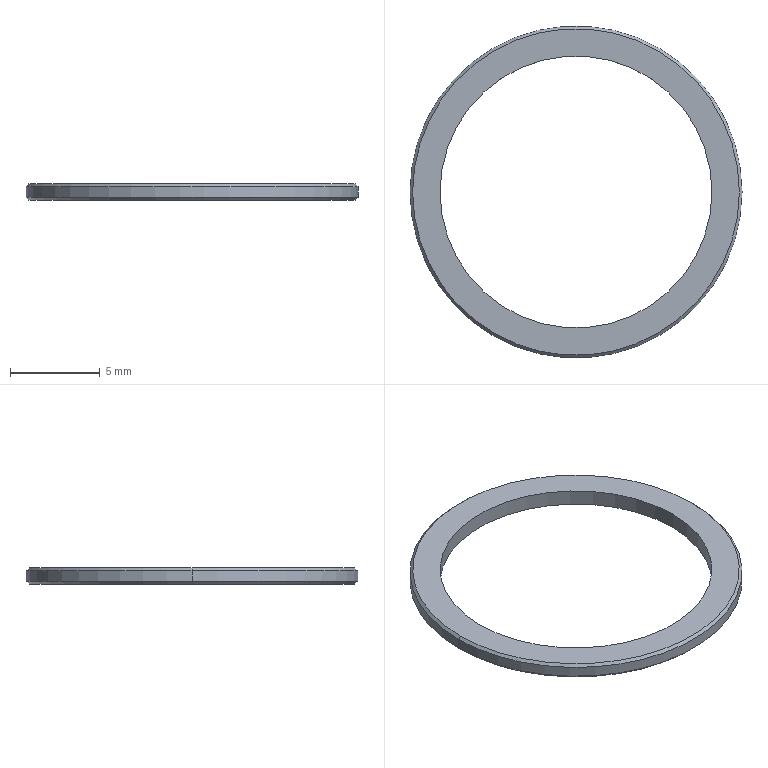Part | STEP file | ARANDELA INT. RODAJA | 1 solid | 10 faces | box 18.5 x 18.5 x 0.9 mm | volume 78.382 mm3 | cone 4 | cylinder 4 | plane 2 | commonest cylinder face diameters 15.15 x2 18.5 x2
STEP:
#1=CARTESIAN_POINT('',(9.1,0.,0.9));
#2=VERTEX_POINT('',#1);
#3=CARTESIAN_POINT('',(-9.1,0.,0.9));
#4=VERTEX_POINT('',#3);
#5=CARTESIAN_POINT('',(0.,0.,0.9));
#6=DIRECTION('',(0.,0.,1.));
#7=DIRECTION('',(1.,0.,0.));
#8=AXIS2_PLACEMENT_3D('',#5,#6,#7);
#9=CIRCLE('',#8,9.1);
#10=EDGE_CURVE('',#2,#4,#9,.T.);
#11=ORIENTED_EDGE('',*,*,#10,.F.);
#12=CARTESIAN_POINT('',(9.25,0.,0.75));
#13=VERTEX_POINT('',#12);
#14=CARTESIAN_POINT('',(9.1,0.,0.9));
#15=DIRECTION('',(0.7071,0.,-0.7071));
#16=VECTOR('',#15,1000.);
#17=LINE('',#14,#16);
#18=EDGE_CURVE('',#2,#13,#17,.T.);
#19=ORIENTED_EDGE('',*,*,#18,.T.);
#20=CARTESIAN_POINT('',(-9.25,0.,0.75));
#21=VERTEX_POINT('',#20);
#22=CARTESIAN_POINT('',(0.,0.,0.75));
#23=DIRECTION('',(0.,0.,-1.));
#24=DIRECTION('',(1.,0.,0.));
#25=AXIS2_PLACEMENT_3D('',#22,#23,#24);
#26=CIRCLE('',#25,9.25);
#27=EDGE_CURVE('',#21,#13,#26,.T.);
#28=ORIENTED_EDGE('',*,*,#27,.F.);
#29=CARTESIAN_POINT('',(-9.1,0.,0.9));
#30=DIRECTION('',(-0.7071,0.,-0.7071));
#31=VECTOR('',#30,1000.);
#32=LINE('',#29,#31);
#33=EDGE_CURVE('',#4,#21,#32,.T.);
#34=ORIENTED_EDGE('',*,*,#33,.F.);
#35=EDGE_LOOP('',(#11,#19,#28,#34));
#36=FACE_OUTER_BOUND('',#35,.T.);
#37=CARTESIAN_POINT('',(0.,0.,0.9));
#38=DIRECTION('',(0.,0.,-1.));
#39=DIRECTION('',(-1.,0.,0.));
#40=AXIS2_PLACEMENT_3D('',#37,#38,#39);
#41=CONICAL_SURFACE('',#40,9.1,0.7854);
#42=ADVANCED_FACE('',(#36),#41,.T.);
#43=CARTESIAN_POINT('',(-9.1,0.,0.));
#44=VERTEX_POINT('',#43);
#45=CARTESIAN_POINT('',(9.1,0.,0.));
#46=VERTEX_POINT('',#45);
#47=CARTESIAN_POINT('',(0.,0.,0.));
#48=DIRECTION('',(0.,0.,-1.));
#49=DIRECTION('',(1.,0.,0.));
#50=AXIS2_PLACEMENT_3D('',#47,#48,#49);
#51=CIRCLE('',#50,9.1);
#52=EDGE_CURVE('',#44,#46,#51,.T.);
#53=ORIENTED_EDGE('',*,*,#52,.F.);
#54=CARTESIAN_POINT('',(-9.25,0.,0.15));
#55=VERTEX_POINT('',#54);
#56=CARTESIAN_POINT('',(-9.25,0.,0.15));
#57=DIRECTION('',(-0.7071,0.,0.7071));
#58=VECTOR('',#57,1000.);
#59=LINE('',#56,#58);
#60=EDGE_CURVE('',#44,#55,#59,.T.);
#61=ORIENTED_EDGE('',*,*,#60,.T.);
#62=CARTESIAN_POINT('',(9.25,0.,0.15));
#63=VERTEX_POINT('',#62);
#64=CARTESIAN_POINT('',(0.,0.,0.15));
#65=DIRECTION('',(0.,0.,1.));
#66=DIRECTION('',(1.,0.,0.));
#67=AXIS2_PLACEMENT_3D('',#64,#65,#66);
#68=CIRCLE('',#67,9.25);
#69=EDGE_CURVE('',#63,#55,#68,.T.);
#70=ORIENTED_EDGE('',*,*,#69,.F.);
#71=CARTESIAN_POINT('',(9.25,0.,0.15));
#72=DIRECTION('',(0.7071,0.,0.7071));
#73=VECTOR('',#72,1000.);
#74=LINE('',#71,#73);
#75=EDGE_CURVE('',#46,#63,#74,.T.);
#76=ORIENTED_EDGE('',*,*,#75,.F.);
#77=EDGE_LOOP('',(#53,#61,#70,#76));
#78=FACE_OUTER_BOUND('',#77,.T.);
#79=CARTESIAN_POINT('',(0.,0.,0.15));
#80=DIRECTION('',(0.,0.,1.));
#81=DIRECTION('',(1.,0.,0.));
#82=AXIS2_PLACEMENT_3D('',#79,#80,#81);
#83=CONICAL_SURFACE('',#82,9.25,0.7854);
#84=ADVANCED_FACE('',(#78),#83,.T.);
#85=CARTESIAN_POINT('',(-7.575,0.,0.9));
#86=VERTEX_POINT('',#85);
#87=CARTESIAN_POINT('',(7.575,0.,0.9));
#88=VERTEX_POINT('',#87);
#89=CARTESIAN_POINT('',(0.,0.,0.9));
#90=DIRECTION('',(0.,0.,1.));
#91=DIRECTION('',(1.,0.,0.));
#92=AXIS2_PLACEMENT_3D('',#89,#90,#91);
#93=CIRCLE('',#92,7.575);
#94=EDGE_CURVE('',#86,#88,#93,.T.);
#95=ORIENTED_EDGE('',*,*,#94,.T.);
#96=CARTESIAN_POINT('',(7.575,0.,0.));
#97=VERTEX_POINT('',#96);
#98=CARTESIAN_POINT('',(7.575,0.,0.9));
#99=DIRECTION('',(0.,0.,-1.));
#100=VECTOR('',#99,1000.);
#101=LINE('',#98,#100);
#102=EDGE_CURVE('',#88,#97,#101,.T.);
#103=ORIENTED_EDGE('',*,*,#102,.T.);
#104=CARTESIAN_POINT('',(-7.575,0.,0.));
#105=VERTEX_POINT('',#104);
#106=CARTESIAN_POINT('',(0.,0.,0.));
#107=DIRECTION('',(0.,0.,1.));
#108=DIRECTION('',(1.,0.,0.));
#109=AXIS2_PLACEMENT_3D('',#106,#107,#108);
#110=CIRCLE('',#109,7.575);
#111=EDGE_CURVE('',#105,#97,#110,.T.);
#112=ORIENTED_EDGE('',*,*,#111,.F.);
#113=CARTESIAN_POINT('',(-7.575,0.,0.9));
#114=DIRECTION('',(0.,0.,-1.));
#115=VECTOR('',#114,1000.);
#116=LINE('',#113,#115);
#117=EDGE_CURVE('',#86,#105,#116,.T.);
#118=ORIENTED_EDGE('',*,*,#117,.F.);
#119=EDGE_LOOP('',(#95,#103,#112,#118));
#120=FACE_OUTER_BOUND('',#119,.T.);
#121=CARTESIAN_POINT('',(0.,0.,0.9));
#122=DIRECTION('',(0.,0.,-1.));
#123=DIRECTION('',(-1.,0.,0.));
#124=AXIS2_PLACEMENT_3D('',#121,#122,#123);
#125=CYLINDRICAL_SURFACE('',#124,7.575);
#126=ADVANCED_FACE('',(#120),#125,.F.);
#127=ORIENTED_EDGE('',*,*,#27,.T.);
#128=CARTESIAN_POINT('',(9.25,0.,0.9));
#129=DIRECTION('',(0.,0.,-1.));
#130=VECTOR('',#129,1000.);
#131=LINE('',#128,#130);
#132=EDGE_CURVE('',#13,#63,#131,.T.);
#133=ORIENTED_EDGE('',*,*,#132,.T.);
#134=ORIENTED_EDGE('',*,*,#69,.T.);
#135=CARTESIAN_POINT('',(-9.25,0.,0.9));
#136=DIRECTION('',(0.,0.,-1.));
#137=VECTOR('',#136,1000.);
#138=LINE('',#135,#137);
#139=EDGE_CURVE('',#21,#55,#138,.T.);
#140=ORIENTED_EDGE('',*,*,#139,.F.);
#141=EDGE_LOOP('',(#127,#133,#134,#140));
#142=FACE_OUTER_BOUND('',#141,.T.);
#143=CARTESIAN_POINT('',(0.,0.,0.9));
#144=DIRECTION('',(0.,0.,-1.));
#145=DIRECTION('',(-1.,0.,0.));
#146=AXIS2_PLACEMENT_3D('',#143,#144,#145);
#147=CYLINDRICAL_SURFACE('',#146,9.25);
#148=ADVANCED_FACE('',(#142),#147,.T.);
#149=CARTESIAN_POINT('',(0.,0.,0.9));
#150=DIRECTION('',(0.,0.,1.));
#151=DIRECTION('',(1.,0.,0.));
#152=AXIS2_PLACEMENT_3D('',#149,#150,#151);
#153=CIRCLE('',#152,9.1);
#154=EDGE_CURVE('',#4,#2,#153,.T.);
#155=ORIENTED_EDGE('',*,*,#154,.T.);
#156=ORIENTED_EDGE('',*,*,#10,.T.);
#157=EDGE_LOOP('',(#155,#156));
#158=FACE_OUTER_BOUND('',#157,.T.);
#159=ORIENTED_EDGE('',*,*,#94,.F.);
#160=CARTESIAN_POINT('',(0.,0.,0.9));
#161=DIRECTION('',(0.,0.,1.));
#162=DIRECTION('',(1.,0.,0.));
#163=AXIS2_PLACEMENT_3D('',#160,#161,#162);
#164=CIRCLE('',#163,7.575);
#165=EDGE_CURVE('',#88,#86,#164,.T.);
#166=ORIENTED_EDGE('',*,*,#165,.F.);
#167=EDGE_LOOP('',(#159,#166));
#168=FACE_BOUND('',#167,.T.);
#169=CARTESIAN_POINT('',(0.,0.,0.9));
#170=DIRECTION('',(0.,0.,1.));
#171=DIRECTION('',(1.,0.,0.));
#172=AXIS2_PLACEMENT_3D('',#169,#170,#171);
#173=PLANE('',#172);
#174=ADVANCED_FACE('',(#158,#168),#173,.T.);
#175=CARTESIAN_POINT('',(0.,0.,0.));
#176=DIRECTION('',(0.,0.,-1.));
#177=DIRECTION('',(1.,0.,0.));
#178=AXIS2_PLACEMENT_3D('',#175,#176,#177);
#179=CIRCLE('',#178,9.1);
#180=EDGE_CURVE('',#46,#44,#179,.T.);
#181=ORIENTED_EDGE('',*,*,#180,.T.);
#182=ORIENTED_EDGE('',*,*,#52,.T.);
#183=EDGE_LOOP('',(#181,#182));
#184=FACE_OUTER_BOUND('',#183,.T.);
#185=ORIENTED_EDGE('',*,*,#111,.T.);
#186=CARTESIAN_POINT('',(0.,0.,0.));
#187=DIRECTION('',(0.,0.,1.));
#188=DIRECTION('',(1.,0.,0.));
#189=AXIS2_PLACEMENT_3D('',#186,#187,#188);
#190=CIRCLE('',#189,7.575);
#191=EDGE_CURVE('',#97,#105,#190,.T.);
#192=ORIENTED_EDGE('',*,*,#191,.T.);
#193=EDGE_LOOP('',(#185,#192));
#194=FACE_BOUND('',#193,.T.);
#195=CARTESIAN_POINT('',(0.,0.,0.));
#196=DIRECTION('',(0.,0.,1.));
#197=DIRECTION('',(1.,0.,0.));
#198=AXIS2_PLACEMENT_3D('',#195,#196,#197);
#199=PLANE('',#198);
#200=ADVANCED_FACE('',(#184,#194),#199,.F.);
#201=ORIENTED_EDGE('',*,*,#132,.F.);
#202=CARTESIAN_POINT('',(0.,0.,0.75));
#203=DIRECTION('',(0.,0.,-1.));
#204=DIRECTION('',(1.,0.,0.));
#205=AXIS2_PLACEMENT_3D('',#202,#203,#204);
#206=CIRCLE('',#205,9.25);
#207=EDGE_CURVE('',#13,#21,#206,.T.);
#208=ORIENTED_EDGE('',*,*,#207,.T.);
#209=ORIENTED_EDGE('',*,*,#139,.T.);
#210=CARTESIAN_POINT('',(0.,0.,0.15));
#211=DIRECTION('',(0.,0.,1.));
#212=DIRECTION('',(1.,0.,0.));
#213=AXIS2_PLACEMENT_3D('',#210,#211,#212);
#214=CIRCLE('',#213,9.25);
#215=EDGE_CURVE('',#55,#63,#214,.T.);
#216=ORIENTED_EDGE('',*,*,#215,.T.);
#217=EDGE_LOOP('',(#201,#208,#209,#216));
#218=FACE_OUTER_BOUND('',#217,.T.);
#219=CARTESIAN_POINT('',(0.,0.,0.9));
#220=DIRECTION('',(0.,0.,-1.));
#221=DIRECTION('',(-1.,0.,0.));
#222=AXIS2_PLACEMENT_3D('',#219,#220,#221);
#223=CYLINDRICAL_SURFACE('',#222,9.25);
#224=ADVANCED_FACE('',(#218),#223,.T.);
#225=ORIENTED_EDGE('',*,*,#102,.F.);
#226=ORIENTED_EDGE('',*,*,#165,.T.);
#227=ORIENTED_EDGE('',*,*,#117,.T.);
#228=ORIENTED_EDGE('',*,*,#191,.F.);
#229=EDGE_LOOP('',(#225,#226,#227,#228));
#230=FACE_OUTER_BOUND('',#229,.T.);
#231=CARTESIAN_POINT('',(0.,0.,0.9));
#232=DIRECTION('',(0.,0.,-1.));
#233=DIRECTION('',(-1.,0.,0.));
#234=AXIS2_PLACEMENT_3D('',#231,#232,#233);
#235=CYLINDRICAL_SURFACE('',#234,7.575);
#236=ADVANCED_FACE('',(#230),#235,.F.);
#237=ORIENTED_EDGE('',*,*,#60,.F.);
#238=ORIENTED_EDGE('',*,*,#180,.F.);
#239=ORIENTED_EDGE('',*,*,#75,.T.);
#240=ORIENTED_EDGE('',*,*,#215,.F.);
#241=EDGE_LOOP('',(#237,#238,#239,#240));
#242=FACE_OUTER_BOUND('',#241,.T.);
#243=CARTESIAN_POINT('',(0.,0.,0.15));
#244=DIRECTION('',(0.,0.,1.));
#245=DIRECTION('',(1.,0.,0.));
#246=AXIS2_PLACEMENT_3D('',#243,#244,#245);
#247=CONICAL_SURFACE('',#246,9.25,0.7854);
#248=ADVANCED_FACE('',(#242),#247,.T.);
#249=ORIENTED_EDGE('',*,*,#18,.F.);
#250=ORIENTED_EDGE('',*,*,#154,.F.);
#251=ORIENTED_EDGE('',*,*,#33,.T.);
#252=ORIENTED_EDGE('',*,*,#207,.F.);
#253=EDGE_LOOP('',(#249,#250,#251,#252));
#254=FACE_OUTER_BOUND('',#253,.T.);
#255=CARTESIAN_POINT('',(0.,0.,0.9));
#256=DIRECTION('',(0.,0.,-1.));
#257=DIRECTION('',(-1.,0.,0.));
#258=AXIS2_PLACEMENT_3D('',#255,#256,#257);
#259=CONICAL_SURFACE('',#258,9.1,0.7854);
#260=ADVANCED_FACE('',(#254),#259,.T.);
#261=CLOSED_SHELL('',(#42,#84,#126,#148,#174,#200,#224,#236,#248,#260));
#262=MANIFOLD_SOLID_BREP('',#261);
#263=CARTESIAN_POINT('',(0.,0.,0.));
#264=DIRECTION('',(0.,0.,1.));
#265=DIRECTION('',(1.,0.,0.));
#266=AXIS2_PLACEMENT_3D('',#263,#264,#265);
#267=(LENGTH_UNIT()NAMED_UNIT(*)SI_UNIT(.MILLI.,.METRE.));
#268=UNCERTAINTY_MEASURE_WITH_UNIT(LENGTH_MEASURE(0.00001),#267,'','');
#269=(NAMED_UNIT(*)PLANE_ANGLE_UNIT()SI_UNIT($,.RADIAN.));
#270=(NAMED_UNIT(*)SI_UNIT($,.STERADIAN.)SOLID_ANGLE_UNIT());
#271=(GEOMETRIC_REPRESENTATION_CONTEXT(3)GLOBAL_UNCERTAINTY_ASSIGNED_CONTEXT((#268))GLOBAL_UNIT_ASSIGNED_CONTEXT((#267,#269,#270))REPRESENTATION_CONTEXT('',''));
#272=ADVANCED_BREP_SHAPE_REPRESENTATION('',(#262,#266),#271);